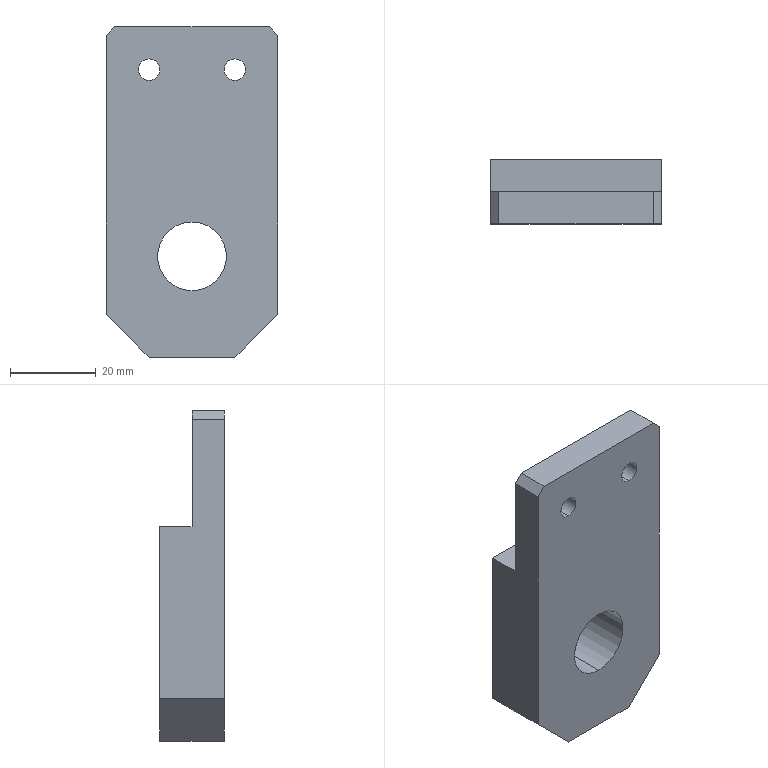Part | STEP file | 0229_219_Arm | 1 solid | 18 faces | box 40 x 15 x 77 mm | volume 33260 mm3 | plane 12 | cylinder 6 | commonest cylinder face diameters 5 x4 16 x2
STEP:
#1=CARTESIAN_POINT('',(0.,0.,0.));
#2=DIRECTION('',(0.,0.,1.));
#3=DIRECTION('',(1.,0.,0.));
#4=AXIS2_PLACEMENT_3D('',#1,#2,#3);
#5=CARTESIAN_POINT('',(-10.,0.,-7.5));
#6=VERTEX_POINT('',#5);
#7=CARTESIAN_POINT('',(-10.,7.5,-7.5));
#8=VERTEX_POINT('',#7);
#9=CARTESIAN_POINT('',(-10.,7.5,-7.5));
#10=DIRECTION('',(0.,1.,0.));
#11=VECTOR('',#10,1.);
#12=LINE('',#9,#11);
#13=CARTESIAN_POINT('',(-10.,7.5,-10.));
#14=DIRECTION('',(0.,1.,0.));
#15=DIRECTION('',(0.,0.,1.));
#16=AXIS2_PLACEMENT_3D('',#13,#14,#15);
#17=CYLINDRICAL_SURFACE('',#16,2.5);
#18=CARTESIAN_POINT('',(6.283,0.));
#19=DIRECTION('',(0.,1.));
#20=VECTOR('',#19,1.);
#21=LINE('',#18,#20);
#22=(GEOMETRIC_REPRESENTATION_CONTEXT(2)PARAMETRIC_REPRESENTATION_CONTEXT()REPRESENTATION_CONTEXT('',''));
#23=DEFINITIONAL_REPRESENTATION('',(#21),#22);
#24=PCURVE('',#17,#23);
#25=CARTESIAN_POINT('',(-10.,7.5,-10.));
#26=DIRECTION('',(0.,1.,0.));
#27=DIRECTION('',(0.,0.,1.));
#28=AXIS2_PLACEMENT_3D('',#25,#26,#27);
#29=CYLINDRICAL_SURFACE('',#28,2.5);
#30=CARTESIAN_POINT('',(0.,0.));
#31=DIRECTION('',(0.,1.));
#32=VECTOR('',#31,1.);
#33=LINE('',#30,#32);
#34=(GEOMETRIC_REPRESENTATION_CONTEXT(2)PARAMETRIC_REPRESENTATION_CONTEXT()REPRESENTATION_CONTEXT('',''));
#35=DEFINITIONAL_REPRESENTATION('',(#33),#34);
#36=PCURVE('',#29,#35);
#37=SURFACE_CURVE('',#12,(#24,#36),.PCURVE_S1.);
#38=EDGE_CURVE('',#6,#8,#37,.T.);
#39=ORIENTED_EDGE('',*,*,#38,.T.);
#40=CARTESIAN_POINT('',(-10.,7.5,-12.5));
#41=VERTEX_POINT('',#40);
#42=CARTESIAN_POINT('',(-10.,7.5,-10.));
#43=DIRECTION('',(0.,1.,0.));
#44=DIRECTION('',(0.,0.,1.));
#45=AXIS2_PLACEMENT_3D('',#42,#43,#44);
#46=CIRCLE('',#45,2.5);
#47=CARTESIAN_POINT('',(0.,0.));
#48=DIRECTION('',(1.,0.));
#49=VECTOR('',#48,1.);
#50=LINE('',#47,#49);
#51=(GEOMETRIC_REPRESENTATION_CONTEXT(2)PARAMETRIC_REPRESENTATION_CONTEXT()REPRESENTATION_CONTEXT('',''));
#52=DEFINITIONAL_REPRESENTATION('',(#50),#51);
#53=PCURVE('',#17,#52);
#54=CARTESIAN_POINT('',(-20.,7.5,-77.));
#55=DIRECTION('',(0.,-1.,0.));
#56=DIRECTION('',(0.,0.,-1.));
#57=AXIS2_PLACEMENT_3D('',#54,#55,#56);
#58=PLANE('',#57);
#59=CARTESIAN_POINT('',(-69.5,10.));
#60=CARTESIAN_POINT('',(-69.5,14.33));
#61=CARTESIAN_POINT('',(-65.75,12.165));
#62=CARTESIAN_POINT('',(-62.,10.));
#63=CARTESIAN_POINT('',(-65.75,7.835));
#64=CARTESIAN_POINT('',(-69.5,5.67));
#65=CARTESIAN_POINT('',(-69.5,10.));
#66=(BOUNDED_CURVE()B_SPLINE_CURVE(2,(#59,#60,#61,#62,#63,#64,#65),.UNSPECIFIED.,.T.,.F.)B_SPLINE_CURVE_WITH_KNOTS((1,2,2,2,2,1),(-2.094,0.,2.094,4.189,6.283,8.378),.UNSPECIFIED.)CURVE()GEOMETRIC_REPRESENTATION_ITEM()RATIONAL_B_SPLINE_CURVE((1.,0.5,1.,0.5,1.,0.5,1.))REPRESENTATION_ITEM(''));
#67=(GEOMETRIC_REPRESENTATION_CONTEXT(2)PARAMETRIC_REPRESENTATION_CONTEXT()REPRESENTATION_CONTEXT('',''));
#68=DEFINITIONAL_REPRESENTATION('',(#66),#67);
#69=PCURVE('',#58,#68);
#70=SURFACE_CURVE('',#46,(#53,#69),.PCURVE_S1.);
#71=EDGE_CURVE('',#41,#8,#70,.T.);
#72=ORIENTED_EDGE('',*,*,#71,.F.);
#73=CARTESIAN_POINT('',(-10.,0.,-12.5));
#74=VERTEX_POINT('',#73);
#75=CARTESIAN_POINT('',(-10.,7.5,-12.5));
#76=DIRECTION('',(0.,1.,0.));
#77=VECTOR('',#76,1.);
#78=LINE('',#75,#77);
#79=CARTESIAN_POINT('',(3.142,0.));
#80=DIRECTION('',(0.,1.));
#81=VECTOR('',#80,1.);
#82=LINE('',#79,#81);
#83=(GEOMETRIC_REPRESENTATION_CONTEXT(2)PARAMETRIC_REPRESENTATION_CONTEXT()REPRESENTATION_CONTEXT('',''));
#84=DEFINITIONAL_REPRESENTATION('',(#82),#83);
#85=PCURVE('',#17,#84);
#86=CARTESIAN_POINT('',(3.142,0.));
#87=DIRECTION('',(0.,1.));
#88=VECTOR('',#87,1.);
#89=LINE('',#86,#88);
#90=(GEOMETRIC_REPRESENTATION_CONTEXT(2)PARAMETRIC_REPRESENTATION_CONTEXT()REPRESENTATION_CONTEXT('',''));
#91=DEFINITIONAL_REPRESENTATION('',(#89),#90);
#92=PCURVE('',#29,#91);
#93=SURFACE_CURVE('',#78,(#85,#92),.PCURVE_S1.);
#94=EDGE_CURVE('',#74,#41,#93,.T.);
#95=ORIENTED_EDGE('',*,*,#94,.F.);
#96=CARTESIAN_POINT('',(-10.,0.,-10.));
#97=DIRECTION('',(0.,1.,0.));
#98=DIRECTION('',(0.,0.,1.));
#99=AXIS2_PLACEMENT_3D('',#96,#97,#98);
#100=CIRCLE('',#99,2.5);
#101=CARTESIAN_POINT('',(0.,-7.5));
#102=DIRECTION('',(1.,0.));
#103=VECTOR('',#102,1.);
#104=LINE('',#101,#103);
#105=(GEOMETRIC_REPRESENTATION_CONTEXT(2)PARAMETRIC_REPRESENTATION_CONTEXT()REPRESENTATION_CONTEXT('',''));
#106=DEFINITIONAL_REPRESENTATION('',(#104),#105);
#107=PCURVE('',#17,#106);
#108=CARTESIAN_POINT('',(-20.,0.,-77.));
#109=DIRECTION('',(0.,-1.,0.));
#110=DIRECTION('',(0.,0.,-1.));
#111=AXIS2_PLACEMENT_3D('',#108,#109,#110);
#112=PLANE('',#111);
#113=CARTESIAN_POINT('',(-69.5,10.));
#114=CARTESIAN_POINT('',(-69.5,14.33));
#115=CARTESIAN_POINT('',(-65.75,12.165));
#116=CARTESIAN_POINT('',(-62.,10.));
#117=CARTESIAN_POINT('',(-65.75,7.835));
#118=CARTESIAN_POINT('',(-69.5,5.67));
#119=CARTESIAN_POINT('',(-69.5,10.));
#120=(BOUNDED_CURVE()B_SPLINE_CURVE(2,(#113,#114,#115,#116,#117,#118,#119),.UNSPECIFIED.,.T.,.F.)B_SPLINE_CURVE_WITH_KNOTS((1,2,2,2,2,1),(-2.094,0.,2.094,4.189,6.283,8.378),.UNSPECIFIED.)CURVE()GEOMETRIC_REPRESENTATION_ITEM()RATIONAL_B_SPLINE_CURVE((1.,0.5,1.,0.5,1.,0.5,1.))REPRESENTATION_ITEM(''));
#121=(GEOMETRIC_REPRESENTATION_CONTEXT(2)PARAMETRIC_REPRESENTATION_CONTEXT()REPRESENTATION_CONTEXT('',''));
#122=DEFINITIONAL_REPRESENTATION('',(#120),#121);
#123=PCURVE('',#112,#122);
#124=SURFACE_CURVE('',#100,(#107,#123),.PCURVE_S1.);
#125=EDGE_CURVE('',#74,#6,#124,.T.);
#126=ORIENTED_EDGE('',*,*,#125,.T.);
#127=EDGE_LOOP('',(#39,#72,#95,#126));
#128=FACE_BOUND('',#127,.F.);
#129=ADVANCED_FACE('',(#128),#17,.F.);
#130=CARTESIAN_POINT('',(10.,0.,-7.5));
#131=VERTEX_POINT('',#130);
#132=CARTESIAN_POINT('',(10.,7.5,-7.5));
#133=VERTEX_POINT('',#132);
#134=CARTESIAN_POINT('',(10.,7.5,-7.5));
#135=DIRECTION('',(0.,1.,0.));
#136=VECTOR('',#135,1.);
#137=LINE('',#134,#136);
#138=CARTESIAN_POINT('',(10.,7.5,-10.));
#139=DIRECTION('',(0.,1.,0.));
#140=DIRECTION('',(0.,0.,1.));
#141=AXIS2_PLACEMENT_3D('',#138,#139,#140);
#142=CYLINDRICAL_SURFACE('',#141,2.5);
#143=CARTESIAN_POINT('',(6.283,0.));
#144=DIRECTION('',(0.,1.));
#145=VECTOR('',#144,1.);
#146=LINE('',#143,#145);
#147=(GEOMETRIC_REPRESENTATION_CONTEXT(2)PARAMETRIC_REPRESENTATION_CONTEXT()REPRESENTATION_CONTEXT('',''));
#148=DEFINITIONAL_REPRESENTATION('',(#146),#147);
#149=PCURVE('',#142,#148);
#150=CARTESIAN_POINT('',(10.,7.5,-10.));
#151=DIRECTION('',(0.,1.,0.));
#152=DIRECTION('',(0.,0.,1.));
#153=AXIS2_PLACEMENT_3D('',#150,#151,#152);
#154=CYLINDRICAL_SURFACE('',#153,2.5);
#155=CARTESIAN_POINT('',(0.,0.));
#156=DIRECTION('',(0.,1.));
#157=VECTOR('',#156,1.);
#158=LINE('',#155,#157);
#159=(GEOMETRIC_REPRESENTATION_CONTEXT(2)PARAMETRIC_REPRESENTATION_CONTEXT()REPRESENTATION_CONTEXT('',''));
#160=DEFINITIONAL_REPRESENTATION('',(#158),#159);
#161=PCURVE('',#154,#160);
#162=SURFACE_CURVE('',#137,(#149,#161),.PCURVE_S1.);
#163=EDGE_CURVE('',#131,#133,#162,.T.);
#164=ORIENTED_EDGE('',*,*,#163,.T.);
#165=CARTESIAN_POINT('',(10.,7.5,-12.5));
#166=VERTEX_POINT('',#165);
#167=CARTESIAN_POINT('',(10.,7.5,-10.));
#168=DIRECTION('',(0.,1.,0.));
#169=DIRECTION('',(0.,0.,1.));
#170=AXIS2_PLACEMENT_3D('',#167,#168,#169);
#171=CIRCLE('',#170,2.5);
#172=CARTESIAN_POINT('',(0.,0.));
#173=DIRECTION('',(1.,0.));
#174=VECTOR('',#173,1.);
#175=LINE('',#172,#174);
#176=(GEOMETRIC_REPRESENTATION_CONTEXT(2)PARAMETRIC_REPRESENTATION_CONTEXT()REPRESENTATION_CONTEXT('',''));
#177=DEFINITIONAL_REPRESENTATION('',(#175),#176);
#178=PCURVE('',#142,#177);
#179=CARTESIAN_POINT('',(-69.5,30.));
#180=CARTESIAN_POINT('',(-69.5,34.33));
#181=CARTESIAN_POINT('',(-65.75,32.165));
#182=CARTESIAN_POINT('',(-62.,30.));
#183=CARTESIAN_POINT('',(-65.75,27.835));
#184=CARTESIAN_POINT('',(-69.5,25.67));
#185=CARTESIAN_POINT('',(-69.5,30.));
#186=(BOUNDED_CURVE()B_SPLINE_CURVE(2,(#179,#180,#181,#182,#183,#184,#185),.UNSPECIFIED.,.T.,.F.)B_SPLINE_CURVE_WITH_KNOTS((1,2,2,2,2,1),(-2.094,0.,2.094,4.189,6.283,8.378),.UNSPECIFIED.)CURVE()GEOMETRIC_REPRESENTATION_ITEM()RATIONAL_B_SPLINE_CURVE((1.,0.5,1.,0.5,1.,0.5,1.))REPRESENTATION_ITEM(''));
#187=(GEOMETRIC_REPRESENTATION_CONTEXT(2)PARAMETRIC_REPRESENTATION_CONTEXT()REPRESENTATION_CONTEXT('',''));
#188=DEFINITIONAL_REPRESENTATION('',(#186),#187);
#189=PCURVE('',#58,#188);
#190=SURFACE_CURVE('',#171,(#178,#189),.PCURVE_S1.);
#191=EDGE_CURVE('',#166,#133,#190,.T.);
#192=ORIENTED_EDGE('',*,*,#191,.F.);
#193=CARTESIAN_POINT('',(10.,0.,-12.5));
#194=VERTEX_POINT('',#193);
#195=CARTESIAN_POINT('',(10.,7.5,-12.5));
#196=DIRECTION('',(0.,1.,0.));
#197=VECTOR('',#196,1.);
#198=LINE('',#195,#197);
#199=CARTESIAN_POINT('',(3.142,0.));
#200=DIRECTION('',(0.,1.));
#201=VECTOR('',#200,1.);
#202=LINE('',#199,#201);
#203=(GEOMETRIC_REPRESENTATION_CONTEXT(2)PARAMETRIC_REPRESENTATION_CONTEXT()REPRESENTATION_CONTEXT('',''));
#204=DEFINITIONAL_REPRESENTATION('',(#202),#203);
#205=PCURVE('',#142,#204);
#206=CARTESIAN_POINT('',(3.142,0.));
#207=DIRECTION('',(0.,1.));
#208=VECTOR('',#207,1.);
#209=LINE('',#206,#208);
#210=(GEOMETRIC_REPRESENTATION_CONTEXT(2)PARAMETRIC_REPRESENTATION_CONTEXT()REPRESENTATION_CONTEXT('',''));
#211=DEFINITIONAL_REPRESENTATION('',(#209),#210);
#212=PCURVE('',#154,#211);
#213=SURFACE_CURVE('',#198,(#205,#212),.PCURVE_S1.);
#214=EDGE_CURVE('',#194,#166,#213,.T.);
#215=ORIENTED_EDGE('',*,*,#214,.F.);
#216=CARTESIAN_POINT('',(10.,0.,-10.));
#217=DIRECTION('',(0.,1.,0.));
#218=DIRECTION('',(0.,0.,1.));
#219=AXIS2_PLACEMENT_3D('',#216,#217,#218);
#220=CIRCLE('',#219,2.5);
#221=CARTESIAN_POINT('',(0.,-7.5));
#222=DIRECTION('',(1.,0.));
#223=VECTOR('',#222,1.);
#224=LINE('',#221,#223);
#225=(GEOMETRIC_REPRESENTATION_CONTEXT(2)PARAMETRIC_REPRESENTATION_CONTEXT()REPRESENTATION_CONTEXT('',''));
#226=DEFINITIONAL_REPRESENTATION('',(#224),#225);
#227=PCURVE('',#142,#226);
#228=CARTESIAN_POINT('',(-69.5,30.));
#229=CARTESIAN_POINT('',(-69.5,34.33));
#230=CARTESIAN_POINT('',(-65.75,32.165));
#231=CARTESIAN_POINT('',(-62.,30.));
#232=CARTESIAN_POINT('',(-65.75,27.835));
#233=CARTESIAN_POINT('',(-69.5,25.67));
#234=CARTESIAN_POINT('',(-69.5,30.));
#235=(BOUNDED_CURVE()B_SPLINE_CURVE(2,(#228,#229,#230,#231,#232,#233,#234),.UNSPECIFIED.,.T.,.F.)B_SPLINE_CURVE_WITH_KNOTS((1,2,2,2,2,1),(-2.094,0.,2.094,4.189,6.283,8.378),.UNSPECIFIED.)CURVE()GEOMETRIC_REPRESENTATION_ITEM()RATIONAL_B_SPLINE_CURVE((1.,0.5,1.,0.5,1.,0.5,1.))REPRESENTATION_ITEM(''));
#236=(GEOMETRIC_REPRESENTATION_CONTEXT(2)PARAMETRIC_REPRESENTATION_CONTEXT()REPRESENTATION_CONTEXT('',''));
#237=DEFINITIONAL_REPRESENTATION('',(#235),#236);
#238=PCURVE('',#112,#237);
#239=SURFACE_CURVE('',#220,(#227,#238),.PCURVE_S1.);
#240=EDGE_CURVE('',#194,#131,#239,.T.);
#241=ORIENTED_EDGE('',*,*,#240,.T.);
#242=EDGE_LOOP('',(#164,#192,#215,#241));
#243=FACE_BOUND('',#242,.F.);
#244=ADVANCED_FACE('',(#243),#142,.F.);
#245=CARTESIAN_POINT('',(0.,0.,-45.5));
#246=VERTEX_POINT('',#245);
#247=CARTESIAN_POINT('',(0.,15.,-45.5));
#248=VERTEX_POINT('',#247);
#249=CARTESIAN_POINT('',(0.,0.,-45.5));
#250=DIRECTION('',(0.,1.,0.));
#251=VECTOR('',#250,1.);
#252=LINE('',#249,#251);
#253=CARTESIAN_POINT('',(0.,0.,-53.5));
#254=DIRECTION('',(0.,1.,0.));
#255=DIRECTION('',(0.,0.,1.));
#256=AXIS2_PLACEMENT_3D('',#253,#254,#255);
#257=CYLINDRICAL_SURFACE('',#256,8.);
#258=CARTESIAN_POINT('',(6.283,0.));
#259=DIRECTION('',(0.,1.));
#260=VECTOR('',#259,1.);
#261=LINE('',#258,#260);
#262=(GEOMETRIC_REPRESENTATION_CONTEXT(2)PARAMETRIC_REPRESENTATION_CONTEXT()REPRESENTATION_CONTEXT('',''));
#263=DEFINITIONAL_REPRESENTATION('',(#261),#262);
#264=PCURVE('',#257,#263);
#265=CARTESIAN_POINT('',(0.,0.,-53.5));
#266=DIRECTION('',(0.,1.,0.));
#267=DIRECTION('',(0.,0.,1.));
#268=AXIS2_PLACEMENT_3D('',#265,#266,#267);
#269=CYLINDRICAL_SURFACE('',#268,8.);
#270=CARTESIAN_POINT('',(0.,0.));
#271=DIRECTION('',(0.,1.));
#272=VECTOR('',#271,1.);
#273=LINE('',#270,#272);
#274=(GEOMETRIC_REPRESENTATION_CONTEXT(2)PARAMETRIC_REPRESENTATION_CONTEXT()REPRESENTATION_CONTEXT('',''));
#275=DEFINITIONAL_REPRESENTATION('',(#273),#274);
#276=PCURVE('',#269,#275);
#277=SURFACE_CURVE('',#252,(#264,#276),.PCURVE_S1.);
#278=EDGE_CURVE('',#246,#248,#277,.T.);
#279=ORIENTED_EDGE('',*,*,#278,.T.);
#280=CARTESIAN_POINT('',(0.,15.,-61.5));
#281=VERTEX_POINT('',#280);
#282=CARTESIAN_POINT('',(0.,15.,-53.5));
#283=DIRECTION('',(0.,1.,0.));
#284=DIRECTION('',(0.,0.,1.));
#285=AXIS2_PLACEMENT_3D('',#282,#283,#284);
#286=CIRCLE('',#285,8.);
#287=CARTESIAN_POINT('',(0.,15.));
#288=DIRECTION('',(1.,0.));
#289=VECTOR('',#288,1.);
#290=LINE('',#287,#289);
#291=(GEOMETRIC_REPRESENTATION_CONTEXT(2)PARAMETRIC_REPRESENTATION_CONTEXT()REPRESENTATION_CONTEXT('',''));
#292=DEFINITIONAL_REPRESENTATION('',(#290),#291);
#293=PCURVE('',#257,#292);
#294=CARTESIAN_POINT('',(-20.,15.,-77.));
#295=DIRECTION('',(0.,-1.,0.));
#296=DIRECTION('',(0.,0.,-1.));
#297=AXIS2_PLACEMENT_3D('',#294,#295,#296);
#298=PLANE('',#297);
#299=CARTESIAN_POINT('',(-31.5,20.));
#300=CARTESIAN_POINT('',(-31.5,33.856));
#301=CARTESIAN_POINT('',(-19.5,26.928));
#302=CARTESIAN_POINT('',(-7.5,20.));
#303=CARTESIAN_POINT('',(-19.5,13.072));
#304=CARTESIAN_POINT('',(-31.5,6.144));
#305=CARTESIAN_POINT('',(-31.5,20.));
#306=(BOUNDED_CURVE()B_SPLINE_CURVE(2,(#299,#300,#301,#302,#303,#304,#305),.UNSPECIFIED.,.T.,.F.)B_SPLINE_CURVE_WITH_KNOTS((1,2,2,2,2,1),(-2.094,0.,2.094,4.189,6.283,8.378),.UNSPECIFIED.)CURVE()GEOMETRIC_REPRESENTATION_ITEM()RATIONAL_B_SPLINE_CURVE((1.,0.5,1.,0.5,1.,0.5,1.))REPRESENTATION_ITEM(''));
#307=(GEOMETRIC_REPRESENTATION_CONTEXT(2)PARAMETRIC_REPRESENTATION_CONTEXT()REPRESENTATION_CONTEXT('',''));
#308=DEFINITIONAL_REPRESENTATION('',(#306),#307);
#309=PCURVE('',#298,#308);
#310=SURFACE_CURVE('',#286,(#293,#309),.PCURVE_S1.);
#311=EDGE_CURVE('',#281,#248,#310,.T.);
#312=ORIENTED_EDGE('',*,*,#311,.F.);
#313=CARTESIAN_POINT('',(0.,0.,-61.5));
#314=VERTEX_POINT('',#313);
#315=CARTESIAN_POINT('',(0.,0.,-61.5));
#316=DIRECTION('',(0.,1.,0.));
#317=VECTOR('',#316,1.);
#318=LINE('',#315,#317);
#319=CARTESIAN_POINT('',(3.142,0.));
#320=DIRECTION('',(0.,1.));
#321=VECTOR('',#320,1.);
#322=LINE('',#319,#321);
#323=(GEOMETRIC_REPRESENTATION_CONTEXT(2)PARAMETRIC_REPRESENTATION_CONTEXT()REPRESENTATION_CONTEXT('',''));
#324=DEFINITIONAL_REPRESENTATION('',(#322),#323);
#325=PCURVE('',#257,#324);
#326=CARTESIAN_POINT('',(3.142,0.));
#327=DIRECTION('',(0.,1.));
#328=VECTOR('',#327,1.);
#329=LINE('',#326,#328);
#330=(GEOMETRIC_REPRESENTATION_CONTEXT(2)PARAMETRIC_REPRESENTATION_CONTEXT()REPRESENTATION_CONTEXT('',''));
#331=DEFINITIONAL_REPRESENTATION('',(#329),#330);
#332=PCURVE('',#269,#331);
#333=SURFACE_CURVE('',#318,(#325,#332),.PCURVE_S1.);
#334=EDGE_CURVE('',#314,#281,#333,.T.);
#335=ORIENTED_EDGE('',*,*,#334,.F.);
#336=CARTESIAN_POINT('',(0.,0.,-53.5));
#337=DIRECTION('',(0.,1.,0.));
#338=DIRECTION('',(0.,0.,1.));
#339=AXIS2_PLACEMENT_3D('',#336,#337,#338);
#340=CIRCLE('',#339,8.);
#341=CARTESIAN_POINT('',(0.,0.));
#342=DIRECTION('',(1.,0.));
#343=VECTOR('',#342,1.);
#344=LINE('',#341,#343);
#345=(GEOMETRIC_REPRESENTATION_CONTEXT(2)PARAMETRIC_REPRESENTATION_CONTEXT()REPRESENTATION_CONTEXT('',''));
#346=DEFINITIONAL_REPRESENTATION('',(#344),#345);
#347=PCURVE('',#257,#346);
#348=CARTESIAN_POINT('',(-31.5,20.));
#349=CARTESIAN_POINT('',(-31.5,33.856));
#350=CARTESIAN_POINT('',(-19.5,26.928));
#351=CARTESIAN_POINT('',(-7.5,20.));
#352=CARTESIAN_POINT('',(-19.5,13.072));
#353=CARTESIAN_POINT('',(-31.5,6.144));
#354=CARTESIAN_POINT('',(-31.5,20.));
#355=(BOUNDED_CURVE()B_SPLINE_CURVE(2,(#348,#349,#350,#351,#352,#353,#354),.UNSPECIFIED.,.T.,.F.)B_SPLINE_CURVE_WITH_KNOTS((1,2,2,2,2,1),(-2.094,0.,2.094,4.189,6.283,8.378),.UNSPECIFIED.)CURVE()GEOMETRIC_REPRESENTATION_ITEM()RATIONAL_B_SPLINE_CURVE((1.,0.5,1.,0.5,1.,0.5,1.))REPRESENTATION_ITEM(''));
#356=(GEOMETRIC_REPRESENTATION_CONTEXT(2)PARAMETRIC_REPRESENTATION_CONTEXT()REPRESENTATION_CONTEXT('',''));
#357=DEFINITIONAL_REPRESENTATION('',(#355),#356);
#358=PCURVE('',#112,#357);
#359=SURFACE_CURVE('',#340,(#347,#358),.PCURVE_S1.);
#360=EDGE_CURVE('',#314,#246,#359,.T.);
#361=ORIENTED_EDGE('',*,*,#360,.T.);
#362=EDGE_LOOP('',(#279,#312,#335,#361));
#363=FACE_BOUND('',#362,.F.);
#364=ADVANCED_FACE('',(#363),#257,.F.);
#365=CARTESIAN_POINT('',(-20.,0.,-67.));
#366=VERTEX_POINT('',#365);
#367=CARTESIAN_POINT('',(-20.,0.,-2.));
#368=VERTEX_POINT('',#367);
#369=CARTESIAN_POINT('',(-20.,0.,0.));
#370=DIRECTION('',(0.,0.,1.));
#371=VECTOR('',#370,1.);
#372=LINE('',#369,#371);
#373=CARTESIAN_POINT('',(-20.,15.,0.));
#374=DIRECTION('',(1.,0.,0.));
#375=DIRECTION('',(0.,0.,-1.));
#376=AXIS2_PLACEMENT_3D('',#373,#374,#375);
#377=PLANE('',#376);
#378=CARTESIAN_POINT('',(0.,-15.));
#379=DIRECTION('',(-1.,0.));
#380=VECTOR('',#379,1.);
#381=LINE('',#378,#380);
#382=(GEOMETRIC_REPRESENTATION_CONTEXT(2)PARAMETRIC_REPRESENTATION_CONTEXT()REPRESENTATION_CONTEXT('',''));
#383=DEFINITIONAL_REPRESENTATION('',(#381),#382);
#384=PCURVE('',#377,#383);
#385=CARTESIAN_POINT('',(-77.,0.));
#386=DIRECTION('',(-1.,0.));
#387=VECTOR('',#386,1.);
#388=LINE('',#385,#387);
#389=(GEOMETRIC_REPRESENTATION_CONTEXT(2)PARAMETRIC_REPRESENTATION_CONTEXT()REPRESENTATION_CONTEXT('',''));
#390=DEFINITIONAL_REPRESENTATION('',(#388),#389);
#391=PCURVE('',#112,#390);
#392=SURFACE_CURVE('',#372,(#384,#391),.PCURVE_S1.);
#393=EDGE_CURVE('',#366,#368,#392,.T.);
#394=ORIENTED_EDGE('',*,*,#393,.T.);
#395=CARTESIAN_POINT('',(-20.,7.5,-2.));
#396=VERTEX_POINT('',#395);
#397=CARTESIAN_POINT('',(-20.,15.,-2.));
#398=DIRECTION('',(0.,1.,0.));
#399=VECTOR('',#398,1.);
#400=LINE('',#397,#399);
#401=CARTESIAN_POINT('',(2.,0.));
#402=DIRECTION('',(0.,1.));
#403=VECTOR('',#402,1.);
#404=LINE('',#401,#403);
#405=(GEOMETRIC_REPRESENTATION_CONTEXT(2)PARAMETRIC_REPRESENTATION_CONTEXT()REPRESENTATION_CONTEXT('',''));
#406=DEFINITIONAL_REPRESENTATION('',(#404),#405);
#407=PCURVE('',#377,#406);
#408=CARTESIAN_POINT('',(-18.,15.,0.));
#409=DIRECTION('',(0.7071,0.,-0.7071));
#410=DIRECTION('',(-0.7071,0.,-0.7071));
#411=AXIS2_PLACEMENT_3D('',#408,#409,#410);
#412=PLANE('',#411);
#413=CARTESIAN_POINT('',(2.828,0.));
#414=DIRECTION('',(0.,1.));
#415=VECTOR('',#414,1.);
#416=LINE('',#413,#415);
#417=(GEOMETRIC_REPRESENTATION_CONTEXT(2)PARAMETRIC_REPRESENTATION_CONTEXT()REPRESENTATION_CONTEXT('',''));
#418=DEFINITIONAL_REPRESENTATION('',(#416),#417);
#419=PCURVE('',#412,#418);
#420=SURFACE_CURVE('',#400,(#407,#419),.PCURVE_S1.);
#421=EDGE_CURVE('',#368,#396,#420,.T.);
#422=ORIENTED_EDGE('',*,*,#421,.T.);
#423=CARTESIAN_POINT('',(-20.,7.5,-27.));
#424=VERTEX_POINT('',#423);
#425=CARTESIAN_POINT('',(-20.,7.5,0.));
#426=DIRECTION('',(0.,0.,1.));
#427=VECTOR('',#426,1.);
#428=LINE('',#425,#427);
#429=CARTESIAN_POINT('',(0.,-7.5));
#430=DIRECTION('',(-1.,0.));
#431=VECTOR('',#430,1.);
#432=LINE('',#429,#431);
#433=(GEOMETRIC_REPRESENTATION_CONTEXT(2)PARAMETRIC_REPRESENTATION_CONTEXT()REPRESENTATION_CONTEXT('',''));
#434=DEFINITIONAL_REPRESENTATION('',(#432),#433);
#435=PCURVE('',#377,#434);
#436=CARTESIAN_POINT('',(-77.,0.));
#437=DIRECTION('',(-1.,0.));
#438=VECTOR('',#437,1.);
#439=LINE('',#436,#438);
#440=(GEOMETRIC_REPRESENTATION_CONTEXT(2)PARAMETRIC_REPRESENTATION_CONTEXT()REPRESENTATION_CONTEXT('',''));
#441=DEFINITIONAL_REPRESENTATION('',(#439),#440);
#442=PCURVE('',#58,#441);
#443=SURFACE_CURVE('',#428,(#435,#442),.PCURVE_S1.);
#444=EDGE_CURVE('',#424,#396,#443,.T.);
#445=ORIENTED_EDGE('',*,*,#444,.F.);
#446=CARTESIAN_POINT('',(-20.,15.,-27.));
#447=VERTEX_POINT('',#446);
#448=CARTESIAN_POINT('',(-20.,-48.26,-27.));
#449=DIRECTION('',(0.,1.,0.));
#450=VECTOR('',#449,1.);
#451=LINE('',#448,#450);
#452=CARTESIAN_POINT('',(27.,-63.26));
#453=DIRECTION('',(0.,1.));
#454=VECTOR('',#453,1.);
#455=LINE('',#452,#454);
#456=(GEOMETRIC_REPRESENTATION_CONTEXT(2)PARAMETRIC_REPRESENTATION_CONTEXT()REPRESENTATION_CONTEXT('',''));
#457=DEFINITIONAL_REPRESENTATION('',(#455),#456);
#458=PCURVE('',#377,#457);
#459=CARTESIAN_POINT('',(-20.,-48.26,-27.));
#460=DIRECTION('',(0.,0.,-1.));
#461=DIRECTION('',(-1.,0.,0.));
#462=AXIS2_PLACEMENT_3D('',#459,#460,#461);
#463=PLANE('',#462);
#464=CARTESIAN_POINT('',(0.,0.));
#465=DIRECTION('',(0.,1.));
#466=VECTOR('',#465,1.);
#467=LINE('',#464,#466);
#468=(GEOMETRIC_REPRESENTATION_CONTEXT(2)PARAMETRIC_REPRESENTATION_CONTEXT()REPRESENTATION_CONTEXT('',''));
#469=DEFINITIONAL_REPRESENTATION('',(#467),#468);
#470=PCURVE('',#463,#469);
#471=SURFACE_CURVE('',#451,(#458,#470),.PCURVE_S1.);
#472=EDGE_CURVE('',#424,#447,#471,.T.);
#473=ORIENTED_EDGE('',*,*,#472,.T.);
#474=CARTESIAN_POINT('',(-20.,15.,-67.));
#475=VERTEX_POINT('',#474);
#476=CARTESIAN_POINT('',(-20.,15.,0.));
#477=DIRECTION('',(0.,0.,1.));
#478=VECTOR('',#477,1.);
#479=LINE('',#476,#478);
#480=CARTESIAN_POINT('',(0.,0.));
#481=DIRECTION('',(-1.,0.));
#482=VECTOR('',#481,1.);
#483=LINE('',#480,#482);
#484=(GEOMETRIC_REPRESENTATION_CONTEXT(2)PARAMETRIC_REPRESENTATION_CONTEXT()REPRESENTATION_CONTEXT('',''));
#485=DEFINITIONAL_REPRESENTATION('',(#483),#484);
#486=PCURVE('',#377,#485);
#487=CARTESIAN_POINT('',(-77.,0.));
#488=DIRECTION('',(-1.,0.));
#489=VECTOR('',#488,1.);
#490=LINE('',#487,#489);
#491=(GEOMETRIC_REPRESENTATION_CONTEXT(2)PARAMETRIC_REPRESENTATION_CONTEXT()REPRESENTATION_CONTEXT('',''));
#492=DEFINITIONAL_REPRESENTATION('',(#490),#491);
#493=PCURVE('',#298,#492);
#494=SURFACE_CURVE('',#479,(#486,#493),.PCURVE_S1.);
#495=EDGE_CURVE('',#475,#447,#494,.T.);
#496=ORIENTED_EDGE('',*,*,#495,.F.);
#497=CARTESIAN_POINT('',(-20.,15.,-67.));
#498=DIRECTION('',(0.,-1.,0.));
#499=VECTOR('',#498,1.);
#500=LINE('',#497,#499);
#501=CARTESIAN_POINT('',(67.,0.));
#502=DIRECTION('',(0.,-1.));
#503=VECTOR('',#502,1.);
#504=LINE('',#501,#503);
#505=(GEOMETRIC_REPRESENTATION_CONTEXT(2)PARAMETRIC_REPRESENTATION_CONTEXT()REPRESENTATION_CONTEXT('',''));
#506=DEFINITIONAL_REPRESENTATION('',(#504),#505);
#507=PCURVE('',#377,#506);
#508=CARTESIAN_POINT('',(-20.,15.,-67.));
#509=DIRECTION('',(0.7071,0.,0.7071));
#510=DIRECTION('',(0.7071,0.,-0.7071));
#511=AXIS2_PLACEMENT_3D('',#508,#509,#510);
#512=PLANE('',#511);
#513=CARTESIAN_POINT('',(0.,0.));
#514=DIRECTION('',(0.,-1.));
#515=VECTOR('',#514,1.);
#516=LINE('',#513,#515);
#517=(GEOMETRIC_REPRESENTATION_CONTEXT(2)PARAMETRIC_REPRESENTATION_CONTEXT()REPRESENTATION_CONTEXT('',''));
#518=DEFINITIONAL_REPRESENTATION('',(#516),#517);
#519=PCURVE('',#512,#518);
#520=SURFACE_CURVE('',#500,(#507,#519),.PCURVE_S1.);
#521=EDGE_CURVE('',#475,#366,#520,.T.);
#522=ORIENTED_EDGE('',*,*,#521,.T.);
#523=EDGE_LOOP('',(#394,#422,#445,#473,#496,#522));
#524=FACE_BOUND('',#523,.T.);
#525=ADVANCED_FACE('',(#524),#377,.F.);
#526=CARTESIAN_POINT('',(-18.,0.,0.));
#527=VERTEX_POINT('',#526);
#528=CARTESIAN_POINT('',(18.,0.,0.));
#529=VERTEX_POINT('',#528);
#530=CARTESIAN_POINT('',(-20.,0.,0.));
#531=DIRECTION('',(1.,0.,0.));
#532=VECTOR('',#531,1.);
#533=LINE('',#530,#532);
#534=CARTESIAN_POINT('',(-20.,15.,0.));
#535=DIRECTION('',(0.,0.,-1.));
#536=DIRECTION('',(-1.,0.,0.));
#537=AXIS2_PLACEMENT_3D('',#534,#535,#536);
#538=PLANE('',#537);
#539=CARTESIAN_POINT('',(0.,-15.));
#540=DIRECTION('',(-1.,0.));
#541=VECTOR('',#540,1.);
#542=LINE('',#539,#541);
#543=(GEOMETRIC_REPRESENTATION_CONTEXT(2)PARAMETRIC_REPRESENTATION_CONTEXT()REPRESENTATION_CONTEXT('',''));
#544=DEFINITIONAL_REPRESENTATION('',(#542),#543);
#545=PCURVE('',#538,#544);
#546=CARTESIAN_POINT('',(-77.,0.));
#547=DIRECTION('',(0.,1.));
#548=VECTOR('',#547,1.);
#549=LINE('',#546,#548);
#550=(GEOMETRIC_REPRESENTATION_CONTEXT(2)PARAMETRIC_REPRESENTATION_CONTEXT()REPRESENTATION_CONTEXT('',''));
#551=DEFINITIONAL_REPRESENTATION('',(#549),#550);
#552=PCURVE('',#112,#551);
#553=SURFACE_CURVE('',#533,(#545,#552),.PCURVE_S1.);
#554=EDGE_CURVE('',#527,#529,#553,.T.);
#555=ORIENTED_EDGE('',*,*,#554,.T.);
#556=CARTESIAN_POINT('',(18.,7.5,0.));
#557=VERTEX_POINT('',#556);
#558=CARTESIAN_POINT('',(18.,15.,0.));
#559=DIRECTION('',(0.,1.,0.));
#560=VECTOR('',#559,1.);
#561=LINE('',#558,#560);
#562=CARTESIAN_POINT('',(-38.,0.));
#563=DIRECTION('',(0.,1.));
#564=VECTOR('',#563,1.);
#565=LINE('',#562,#564);
#566=(GEOMETRIC_REPRESENTATION_CONTEXT(2)PARAMETRIC_REPRESENTATION_CONTEXT()REPRESENTATION_CONTEXT('',''));
#567=DEFINITIONAL_REPRESENTATION('',(#565),#566);
#568=PCURVE('',#538,#567);
#569=CARTESIAN_POINT('',(20.,15.,-2.));
#570=DIRECTION('',(-0.7071,0.,-0.7071));
#571=DIRECTION('',(-0.7071,0.,0.7071));
#572=AXIS2_PLACEMENT_3D('',#569,#570,#571);
#573=PLANE('',#572);
#574=CARTESIAN_POINT('',(2.828,0.));
#575=DIRECTION('',(0.,1.));
#576=VECTOR('',#575,1.);
#577=LINE('',#574,#576);
#578=(GEOMETRIC_REPRESENTATION_CONTEXT(2)PARAMETRIC_REPRESENTATION_CONTEXT()REPRESENTATION_CONTEXT('',''));
#579=DEFINITIONAL_REPRESENTATION('',(#577),#578);
#580=PCURVE('',#573,#579);
#581=SURFACE_CURVE('',#561,(#568,#580),.PCURVE_S1.);
#582=EDGE_CURVE('',#529,#557,#581,.T.);
#583=ORIENTED_EDGE('',*,*,#582,.T.);
#584=CARTESIAN_POINT('',(-18.,7.5,0.));
#585=VERTEX_POINT('',#584);
#586=CARTESIAN_POINT('',(-20.,7.5,0.));
#587=DIRECTION('',(1.,0.,0.));
#588=VECTOR('',#587,1.);
#589=LINE('',#586,#588);
#590=CARTESIAN_POINT('',(0.,-7.5));
#591=DIRECTION('',(-1.,0.));
#592=VECTOR('',#591,1.);
#593=LINE('',#590,#592);
#594=(GEOMETRIC_REPRESENTATION_CONTEXT(2)PARAMETRIC_REPRESENTATION_CONTEXT()REPRESENTATION_CONTEXT('',''));
#595=DEFINITIONAL_REPRESENTATION('',(#593),#594);
#596=PCURVE('',#538,#595);
#597=CARTESIAN_POINT('',(-77.,0.));
#598=DIRECTION('',(0.,1.));
#599=VECTOR('',#598,1.);
#600=LINE('',#597,#599);
#601=(GEOMETRIC_REPRESENTATION_CONTEXT(2)PARAMETRIC_REPRESENTATION_CONTEXT()REPRESENTATION_CONTEXT('',''));
#602=DEFINITIONAL_REPRESENTATION('',(#600),#601);
#603=PCURVE('',#58,#602);
#604=SURFACE_CURVE('',#589,(#596,#603),.PCURVE_S1.);
#605=EDGE_CURVE('',#585,#557,#604,.T.);
#606=ORIENTED_EDGE('',*,*,#605,.F.);
#607=CARTESIAN_POINT('',(-18.,15.,0.));
#608=DIRECTION('',(0.,-1.,0.));
#609=VECTOR('',#608,1.);
#610=LINE('',#607,#609);
#611=CARTESIAN_POINT('',(-2.,0.));
#612=DIRECTION('',(0.,-1.));
#613=VECTOR('',#612,1.);
#614=LINE('',#611,#613);
#615=(GEOMETRIC_REPRESENTATION_CONTEXT(2)PARAMETRIC_REPRESENTATION_CONTEXT()REPRESENTATION_CONTEXT('',''));
#616=DEFINITIONAL_REPRESENTATION('',(#614),#615);
#617=PCURVE('',#538,#616);
#618=CARTESIAN_POINT('',(0.,0.));
#619=DIRECTION('',(0.,-1.));
#620=VECTOR('',#619,1.);
#621=LINE('',#618,#620);
#622=(GEOMETRIC_REPRESENTATION_CONTEXT(2)PARAMETRIC_REPRESENTATION_CONTEXT()REPRESENTATION_CONTEXT('',''));
#623=DEFINITIONAL_REPRESENTATION('',(#621),#622);
#624=PCURVE('',#412,#623);
#625=SURFACE_CURVE('',#610,(#617,#624),.PCURVE_S1.);
#626=EDGE_CURVE('',#585,#527,#625,.T.);
#627=ORIENTED_EDGE('',*,*,#626,.T.);
#628=EDGE_LOOP('',(#555,#583,#606,#627));
#629=FACE_BOUND('',#628,.T.);
#630=ADVANCED_FACE('',(#629),#538,.F.);
#631=CARTESIAN_POINT('',(20.,7.5,-2.));
#632=VERTEX_POINT('',#631);
#633=CARTESIAN_POINT('',(20.,7.5,-27.));
#634=VERTEX_POINT('',#633);
#635=CARTESIAN_POINT('',(20.,7.5,0.));
#636=DIRECTION('',(0.,0.,-1.));
#637=VECTOR('',#636,1.);
#638=LINE('',#635,#637);
#639=CARTESIAN_POINT('',(20.,15.,0.));
#640=DIRECTION('',(-1.,0.,0.));
#641=DIRECTION('',(0.,0.,1.));
#642=AXIS2_PLACEMENT_3D('',#639,#640,#641);
#643=PLANE('',#642);
#644=CARTESIAN_POINT('',(0.,-7.5));
#645=DIRECTION('',(-1.,0.));
#646=VECTOR('',#645,1.);
#647=LINE('',#644,#646);
#648=(GEOMETRIC_REPRESENTATION_CONTEXT(2)PARAMETRIC_REPRESENTATION_CONTEXT()REPRESENTATION_CONTEXT('',''));
#649=DEFINITIONAL_REPRESENTATION('',(#647),#648);
#650=PCURVE('',#643,#649);
#651=CARTESIAN_POINT('',(-77.,40.));
#652=DIRECTION('',(1.,0.));
#653=VECTOR('',#652,1.);
#654=LINE('',#651,#653);
#655=(GEOMETRIC_REPRESENTATION_CONTEXT(2)PARAMETRIC_REPRESENTATION_CONTEXT()REPRESENTATION_CONTEXT('',''));
#656=DEFINITIONAL_REPRESENTATION('',(#654),#655);
#657=PCURVE('',#58,#656);
#658=SURFACE_CURVE('',#638,(#650,#657),.PCURVE_S1.);
#659=EDGE_CURVE('',#632,#634,#658,.T.);
#660=ORIENTED_EDGE('',*,*,#659,.F.);
#661=CARTESIAN_POINT('',(20.,0.,-2.));
#662=VERTEX_POINT('',#661);
#663=CARTESIAN_POINT('',(20.,15.,-2.));
#664=DIRECTION('',(0.,-1.,0.));
#665=VECTOR('',#664,1.);
#666=LINE('',#663,#665);
#667=CARTESIAN_POINT('',(-2.,0.));
#668=DIRECTION('',(0.,-1.));
#669=VECTOR('',#668,1.);
#670=LINE('',#667,#669);
#671=(GEOMETRIC_REPRESENTATION_CONTEXT(2)PARAMETRIC_REPRESENTATION_CONTEXT()REPRESENTATION_CONTEXT('',''));
#672=DEFINITIONAL_REPRESENTATION('',(#670),#671);
#673=PCURVE('',#643,#672);
#674=CARTESIAN_POINT('',(0.,0.));
#675=DIRECTION('',(0.,-1.));
#676=VECTOR('',#675,1.);
#677=LINE('',#674,#676);
#678=(GEOMETRIC_REPRESENTATION_CONTEXT(2)PARAMETRIC_REPRESENTATION_CONTEXT()REPRESENTATION_CONTEXT('',''));
#679=DEFINITIONAL_REPRESENTATION('',(#677),#678);
#680=PCURVE('',#573,#679);
#681=SURFACE_CURVE('',#666,(#673,#680),.PCURVE_S1.);
#682=EDGE_CURVE('',#632,#662,#681,.T.);
#683=ORIENTED_EDGE('',*,*,#682,.T.);
#684=CARTESIAN_POINT('',(20.,0.,-67.));
#685=VERTEX_POINT('',#684);
#686=CARTESIAN_POINT('',(20.,0.,0.));
#687=DIRECTION('',(0.,0.,-1.));
#688=VECTOR('',#687,1.);
#689=LINE('',#686,#688);
#690=CARTESIAN_POINT('',(0.,-15.));
#691=DIRECTION('',(-1.,0.));
#692=VECTOR('',#691,1.);
#693=LINE('',#690,#692);
#694=(GEOMETRIC_REPRESENTATION_CONTEXT(2)PARAMETRIC_REPRESENTATION_CONTEXT()REPRESENTATION_CONTEXT('',''));
#695=DEFINITIONAL_REPRESENTATION('',(#693),#694);
#696=PCURVE('',#643,#695);
#697=CARTESIAN_POINT('',(-77.,40.));
#698=DIRECTION('',(1.,0.));
#699=VECTOR('',#698,1.);
#700=LINE('',#697,#699);
#701=(GEOMETRIC_REPRESENTATION_CONTEXT(2)PARAMETRIC_REPRESENTATION_CONTEXT()REPRESENTATION_CONTEXT('',''));
#702=DEFINITIONAL_REPRESENTATION('',(#700),#701);
#703=PCURVE('',#112,#702);
#704=SURFACE_CURVE('',#689,(#696,#703),.PCURVE_S1.);
#705=EDGE_CURVE('',#662,#685,#704,.T.);
#706=ORIENTED_EDGE('',*,*,#705,.T.);
#707=CARTESIAN_POINT('',(20.,15.,-67.));
#708=VERTEX_POINT('',#707);
#709=CARTESIAN_POINT('',(20.,15.,-67.));
#710=DIRECTION('',(0.,1.,0.));
#711=VECTOR('',#710,1.);
#712=LINE('',#709,#711);
#713=CARTESIAN_POINT('',(-67.,0.));
#714=DIRECTION('',(0.,1.));
#715=VECTOR('',#714,1.);
#716=LINE('',#713,#715);
#717=(GEOMETRIC_REPRESENTATION_CONTEXT(2)PARAMETRIC_REPRESENTATION_CONTEXT()REPRESENTATION_CONTEXT('',''));
#718=DEFINITIONAL_REPRESENTATION('',(#716),#717);
#719=PCURVE('',#643,#718);
#720=CARTESIAN_POINT('',(10.,15.,-77.));
#721=DIRECTION('',(-0.7071,0.,0.7071));
#722=DIRECTION('',(0.7071,0.,0.7071));
#723=AXIS2_PLACEMENT_3D('',#720,#721,#722);
#724=PLANE('',#723);
#725=CARTESIAN_POINT('',(14.142,0.));
#726=DIRECTION('',(0.,1.));
#727=VECTOR('',#726,1.);
#728=LINE('',#725,#727);
#729=(GEOMETRIC_REPRESENTATION_CONTEXT(2)PARAMETRIC_REPRESENTATION_CONTEXT()REPRESENTATION_CONTEXT('',''));
#730=DEFINITIONAL_REPRESENTATION('',(#728),#729);
#731=PCURVE('',#724,#730);
#732=SURFACE_CURVE('',#712,(#719,#731),.PCURVE_S1.);
#733=EDGE_CURVE('',#685,#708,#732,.T.);
#734=ORIENTED_EDGE('',*,*,#733,.T.);
#735=CARTESIAN_POINT('',(20.,15.,-27.));
#736=VERTEX_POINT('',#735);
#737=CARTESIAN_POINT('',(20.,15.,0.));
#738=DIRECTION('',(0.,0.,-1.));
#739=VECTOR('',#738,1.);
#740=LINE('',#737,#739);
#741=CARTESIAN_POINT('',(0.,0.));
#742=DIRECTION('',(-1.,0.));
#743=VECTOR('',#742,1.);
#744=LINE('',#741,#743);
#745=(GEOMETRIC_REPRESENTATION_CONTEXT(2)PARAMETRIC_REPRESENTATION_CONTEXT()REPRESENTATION_CONTEXT('',''));
#746=DEFINITIONAL_REPRESENTATION('',(#744),#745);
#747=PCURVE('',#643,#746);
#748=CARTESIAN_POINT('',(-77.,40.));
#749=DIRECTION('',(1.,0.));
#750=VECTOR('',#749,1.);
#751=LINE('',#748,#750);
#752=(GEOMETRIC_REPRESENTATION_CONTEXT(2)PARAMETRIC_REPRESENTATION_CONTEXT()REPRESENTATION_CONTEXT('',''));
#753=DEFINITIONAL_REPRESENTATION('',(#751),#752);
#754=PCURVE('',#298,#753);
#755=SURFACE_CURVE('',#740,(#747,#754),.PCURVE_S1.);
#756=EDGE_CURVE('',#736,#708,#755,.T.);
#757=ORIENTED_EDGE('',*,*,#756,.F.);
#758=CARTESIAN_POINT('',(20.,-48.26,-27.));
#759=DIRECTION('',(0.,1.,0.));
#760=VECTOR('',#759,1.);
#761=LINE('',#758,#760);
#762=CARTESIAN_POINT('',(-27.,-63.26));
#763=DIRECTION('',(0.,1.));
#764=VECTOR('',#763,1.);
#765=LINE('',#762,#764);
#766=(GEOMETRIC_REPRESENTATION_CONTEXT(2)PARAMETRIC_REPRESENTATION_CONTEXT()REPRESENTATION_CONTEXT('',''));
#767=DEFINITIONAL_REPRESENTATION('',(#765),#766);
#768=PCURVE('',#643,#767);
#769=CARTESIAN_POINT('',(-40.,0.));
#770=DIRECTION('',(0.,1.));
#771=VECTOR('',#770,1.);
#772=LINE('',#769,#771);
#773=(GEOMETRIC_REPRESENTATION_CONTEXT(2)PARAMETRIC_REPRESENTATION_CONTEXT()REPRESENTATION_CONTEXT('',''));
#774=DEFINITIONAL_REPRESENTATION('',(#772),#773);
#775=PCURVE('',#463,#774);
#776=SURFACE_CURVE('',#761,(#768,#775),.PCURVE_S1.);
#777=EDGE_CURVE('',#634,#736,#776,.T.);
#778=ORIENTED_EDGE('',*,*,#777,.F.);
#779=EDGE_LOOP('',(#660,#683,#706,#734,#757,#778));
#780=FACE_BOUND('',#779,.T.);
#781=ADVANCED_FACE('',(#780),#643,.F.);
#782=CARTESIAN_POINT('',(10.,0.,-77.));
#783=VERTEX_POINT('',#782);
#784=CARTESIAN_POINT('',(-10.,0.,-77.));
#785=VERTEX_POINT('',#784);
#786=CARTESIAN_POINT('',(-20.,0.,-77.));
#787=DIRECTION('',(-1.,0.,0.));
#788=VECTOR('',#787,1.);
#789=LINE('',#786,#788);
#790=CARTESIAN_POINT('',(-20.,15.,-77.));
#791=DIRECTION('',(0.,0.,1.));
#792=DIRECTION('',(1.,0.,0.));
#793=AXIS2_PLACEMENT_3D('',#790,#791,#792);
#794=PLANE('',#793);
#795=CARTESIAN_POINT('',(0.,-15.));
#796=DIRECTION('',(-1.,0.));
#797=VECTOR('',#796,1.);
#798=LINE('',#795,#797);
#799=(GEOMETRIC_REPRESENTATION_CONTEXT(2)PARAMETRIC_REPRESENTATION_CONTEXT()REPRESENTATION_CONTEXT('',''));
#800=DEFINITIONAL_REPRESENTATION('',(#798),#799);
#801=PCURVE('',#794,#800);
#802=CARTESIAN_POINT('',(0.,0.));
#803=DIRECTION('',(0.,-1.));
#804=VECTOR('',#803,1.);
#805=LINE('',#802,#804);
#806=(GEOMETRIC_REPRESENTATION_CONTEXT(2)PARAMETRIC_REPRESENTATION_CONTEXT()REPRESENTATION_CONTEXT('',''));
#807=DEFINITIONAL_REPRESENTATION('',(#805),#806);
#808=PCURVE('',#112,#807);
#809=SURFACE_CURVE('',#789,(#801,#808),.PCURVE_S1.);
#810=EDGE_CURVE('',#783,#785,#809,.T.);
#811=ORIENTED_EDGE('',*,*,#810,.T.);
#812=CARTESIAN_POINT('',(-10.,15.,-77.));
#813=VERTEX_POINT('',#812);
#814=CARTESIAN_POINT('',(-10.,15.,-77.));
#815=DIRECTION('',(0.,1.,0.));
#816=VECTOR('',#815,1.);
#817=LINE('',#814,#816);
#818=CARTESIAN_POINT('',(10.,0.));
#819=DIRECTION('',(0.,1.));
#820=VECTOR('',#819,1.);
#821=LINE('',#818,#820);
#822=(GEOMETRIC_REPRESENTATION_CONTEXT(2)PARAMETRIC_REPRESENTATION_CONTEXT()REPRESENTATION_CONTEXT('',''));
#823=DEFINITIONAL_REPRESENTATION('',(#821),#822);
#824=PCURVE('',#794,#823);
#825=CARTESIAN_POINT('',(14.142,0.));
#826=DIRECTION('',(0.,1.));
#827=VECTOR('',#826,1.);
#828=LINE('',#825,#827);
#829=(GEOMETRIC_REPRESENTATION_CONTEXT(2)PARAMETRIC_REPRESENTATION_CONTEXT()REPRESENTATION_CONTEXT('',''));
#830=DEFINITIONAL_REPRESENTATION('',(#828),#829);
#831=PCURVE('',#512,#830);
#832=SURFACE_CURVE('',#817,(#824,#831),.PCURVE_S1.);
#833=EDGE_CURVE('',#785,#813,#832,.T.);
#834=ORIENTED_EDGE('',*,*,#833,.T.);
#835=CARTESIAN_POINT('',(10.,15.,-77.));
#836=VERTEX_POINT('',#835);
#837=CARTESIAN_POINT('',(-20.,15.,-77.));
#838=DIRECTION('',(-1.,0.,0.));
#839=VECTOR('',#838,1.);
#840=LINE('',#837,#839);
#841=CARTESIAN_POINT('',(0.,0.));
#842=DIRECTION('',(-1.,0.));
#843=VECTOR('',#842,1.);
#844=LINE('',#841,#843);
#845=(GEOMETRIC_REPRESENTATION_CONTEXT(2)PARAMETRIC_REPRESENTATION_CONTEXT()REPRESENTATION_CONTEXT('',''));
#846=DEFINITIONAL_REPRESENTATION('',(#844),#845);
#847=PCURVE('',#794,#846);
#848=CARTESIAN_POINT('',(0.,0.));
#849=DIRECTION('',(0.,-1.));
#850=VECTOR('',#849,1.);
#851=LINE('',#848,#850);
#852=(GEOMETRIC_REPRESENTATION_CONTEXT(2)PARAMETRIC_REPRESENTATION_CONTEXT()REPRESENTATION_CONTEXT('',''));
#853=DEFINITIONAL_REPRESENTATION('',(#851),#852);
#854=PCURVE('',#298,#853);
#855=SURFACE_CURVE('',#840,(#847,#854),.PCURVE_S1.);
#856=EDGE_CURVE('',#836,#813,#855,.T.);
#857=ORIENTED_EDGE('',*,*,#856,.F.);
#858=CARTESIAN_POINT('',(10.,15.,-77.));
#859=DIRECTION('',(0.,-1.,0.));
#860=VECTOR('',#859,1.);
#861=LINE('',#858,#860);
#862=CARTESIAN_POINT('',(30.,0.));
#863=DIRECTION('',(0.,-1.));
#864=VECTOR('',#863,1.);
#865=LINE('',#862,#864);
#866=(GEOMETRIC_REPRESENTATION_CONTEXT(2)PARAMETRIC_REPRESENTATION_CONTEXT()REPRESENTATION_CONTEXT('',''));
#867=DEFINITIONAL_REPRESENTATION('',(#865),#866);
#868=PCURVE('',#794,#867);
#869=CARTESIAN_POINT('',(0.,0.));
#870=DIRECTION('',(0.,-1.));
#871=VECTOR('',#870,1.);
#872=LINE('',#869,#871);
#873=(GEOMETRIC_REPRESENTATION_CONTEXT(2)PARAMETRIC_REPRESENTATION_CONTEXT()REPRESENTATION_CONTEXT('',''));
#874=DEFINITIONAL_REPRESENTATION('',(#872),#873);
#875=PCURVE('',#724,#874);
#876=SURFACE_CURVE('',#861,(#868,#875),.PCURVE_S1.);
#877=EDGE_CURVE('',#836,#783,#876,.T.);
#878=ORIENTED_EDGE('',*,*,#877,.T.);
#879=EDGE_LOOP('',(#811,#834,#857,#878));
#880=FACE_BOUND('',#879,.T.);
#881=ADVANCED_FACE('',(#880),#794,.F.);
#882=CARTESIAN_POINT('',(0.,15.,-53.5));
#883=DIRECTION('',(0.,1.,0.));
#884=DIRECTION('',(0.,0.,1.));
#885=AXIS2_PLACEMENT_3D('',#882,#883,#884);
#886=CIRCLE('',#885,8.);
#887=CARTESIAN_POINT('',(-31.5,20.));
#888=CARTESIAN_POINT('',(-31.5,33.856));
#889=CARTESIAN_POINT('',(-19.5,26.928));
#890=CARTESIAN_POINT('',(-7.5,20.));
#891=CARTESIAN_POINT('',(-19.5,13.072));
#892=CARTESIAN_POINT('',(-31.5,6.144));
#893=CARTESIAN_POINT('',(-31.5,20.));
#894=(BOUNDED_CURVE()B_SPLINE_CURVE(2,(#887,#888,#889,#890,#891,#892,#893),.UNSPECIFIED.,.T.,.F.)B_SPLINE_CURVE_WITH_KNOTS((1,2,2,2,2,1),(-2.094,0.,2.094,4.189,6.283,8.378),.UNSPECIFIED.)CURVE()GEOMETRIC_REPRESENTATION_ITEM()RATIONAL_B_SPLINE_CURVE((1.,0.5,1.,0.5,1.,0.5,1.))REPRESENTATION_ITEM(''));
#895=(GEOMETRIC_REPRESENTATION_CONTEXT(2)PARAMETRIC_REPRESENTATION_CONTEXT()REPRESENTATION_CONTEXT('',''));
#896=DEFINITIONAL_REPRESENTATION('',(#894),#895);
#897=PCURVE('',#298,#896);
#898=CARTESIAN_POINT('',(0.,15.));
#899=DIRECTION('',(1.,0.));
#900=VECTOR('',#899,1.);
#901=LINE('',#898,#900);
#902=(GEOMETRIC_REPRESENTATION_CONTEXT(2)PARAMETRIC_REPRESENTATION_CONTEXT()REPRESENTATION_CONTEXT('',''));
#903=DEFINITIONAL_REPRESENTATION('',(#901),#902);
#904=PCURVE('',#269,#903);
#905=SURFACE_CURVE('',#886,(#897,#904),.PCURVE_S1.);
#906=EDGE_CURVE('',#248,#281,#905,.T.);
#907=ORIENTED_EDGE('',*,*,#906,.F.);
#908=ORIENTED_EDGE('',*,*,#311,.F.);
#909=EDGE_LOOP('',(#907,#908));
#910=FACE_BOUND('',#909,.T.);
#911=ORIENTED_EDGE('',*,*,#856,.T.);
#912=CARTESIAN_POINT('',(-20.,15.,-67.));
#913=DIRECTION('',(-0.7071,0.,0.7071));
#914=VECTOR('',#913,1.);
#915=LINE('',#912,#914);
#916=CARTESIAN_POINT('',(-10.,0.));
#917=DIRECTION('',(-0.7071,-0.7071));
#918=VECTOR('',#917,1.);
#919=LINE('',#916,#918);
#920=(GEOMETRIC_REPRESENTATION_CONTEXT(2)PARAMETRIC_REPRESENTATION_CONTEXT()REPRESENTATION_CONTEXT('',''));
#921=DEFINITIONAL_REPRESENTATION('',(#919),#920);
#922=PCURVE('',#298,#921);
#923=CARTESIAN_POINT('',(0.,0.));
#924=DIRECTION('',(-1.,0.));
#925=VECTOR('',#924,1.);
#926=LINE('',#923,#925);
#927=(GEOMETRIC_REPRESENTATION_CONTEXT(2)PARAMETRIC_REPRESENTATION_CONTEXT()REPRESENTATION_CONTEXT('',''));
#928=DEFINITIONAL_REPRESENTATION('',(#926),#927);
#929=PCURVE('',#512,#928);
#930=SURFACE_CURVE('',#915,(#922,#929),.PCURVE_S1.);
#931=EDGE_CURVE('',#813,#475,#930,.T.);
#932=ORIENTED_EDGE('',*,*,#931,.T.);
#933=ORIENTED_EDGE('',*,*,#495,.T.);
#934=CARTESIAN_POINT('',(-20.,15.,-27.));
#935=DIRECTION('',(-1.,0.,0.));
#936=VECTOR('',#935,1.);
#937=LINE('',#934,#936);
#938=CARTESIAN_POINT('',(-50.,0.));
#939=DIRECTION('',(0.,-1.));
#940=VECTOR('',#939,1.);
#941=LINE('',#938,#940);
#942=(GEOMETRIC_REPRESENTATION_CONTEXT(2)PARAMETRIC_REPRESENTATION_CONTEXT()REPRESENTATION_CONTEXT('',''));
#943=DEFINITIONAL_REPRESENTATION('',(#941),#942);
#944=PCURVE('',#298,#943);
#945=CARTESIAN_POINT('',(0.,63.26));
#946=DIRECTION('',(1.,0.));
#947=VECTOR('',#946,1.);
#948=LINE('',#945,#947);
#949=(GEOMETRIC_REPRESENTATION_CONTEXT(2)PARAMETRIC_REPRESENTATION_CONTEXT()REPRESENTATION_CONTEXT('',''));
#950=DEFINITIONAL_REPRESENTATION('',(#948),#949);
#951=PCURVE('',#463,#950);
#952=SURFACE_CURVE('',#937,(#944,#951),.PCURVE_S1.);
#953=EDGE_CURVE('',#736,#447,#952,.T.);
#954=ORIENTED_EDGE('',*,*,#953,.F.);
#955=ORIENTED_EDGE('',*,*,#756,.T.);
#956=CARTESIAN_POINT('',(10.,15.,-77.));
#957=DIRECTION('',(-0.7071,0.,-0.7071));
#958=VECTOR('',#957,1.);
#959=LINE('',#956,#958);
#960=CARTESIAN_POINT('',(0.,30.));
#961=DIRECTION('',(0.7071,-0.7071));
#962=VECTOR('',#961,1.);
#963=LINE('',#960,#962);
#964=(GEOMETRIC_REPRESENTATION_CONTEXT(2)PARAMETRIC_REPRESENTATION_CONTEXT()REPRESENTATION_CONTEXT('',''));
#965=DEFINITIONAL_REPRESENTATION('',(#963),#964);
#966=PCURVE('',#298,#965);
#967=CARTESIAN_POINT('',(0.,0.));
#968=DIRECTION('',(-1.,0.));
#969=VECTOR('',#968,1.);
#970=LINE('',#967,#969);
#971=(GEOMETRIC_REPRESENTATION_CONTEXT(2)PARAMETRIC_REPRESENTATION_CONTEXT()REPRESENTATION_CONTEXT('',''));
#972=DEFINITIONAL_REPRESENTATION('',(#970),#971);
#973=PCURVE('',#724,#972);
#974=SURFACE_CURVE('',#959,(#966,#973),.PCURVE_S1.);
#975=EDGE_CURVE('',#708,#836,#974,.T.);
#976=ORIENTED_EDGE('',*,*,#975,.T.);
#977=EDGE_LOOP('',(#911,#932,#933,#954,#955,#976));
#978=FACE_BOUND('',#977,.T.);
#979=ADVANCED_FACE('',(#910,#978),#298,.F.);
#980=CARTESIAN_POINT('',(-10.,0.,-10.));
#981=DIRECTION('',(0.,1.,0.));
#982=DIRECTION('',(0.,0.,1.));
#983=AXIS2_PLACEMENT_3D('',#980,#981,#982);
#984=CIRCLE('',#983,2.5);
#985=CARTESIAN_POINT('',(-69.5,10.));
#986=CARTESIAN_POINT('',(-69.5,14.33));
#987=CARTESIAN_POINT('',(-65.75,12.165));
#988=CARTESIAN_POINT('',(-62.,10.));
#989=CARTESIAN_POINT('',(-65.75,7.835));
#990=CARTESIAN_POINT('',(-69.5,5.67));
#991=CARTESIAN_POINT('',(-69.5,10.));
#992=(BOUNDED_CURVE()B_SPLINE_CURVE(2,(#985,#986,#987,#988,#989,#990,#991),.UNSPECIFIED.,.T.,.F.)B_SPLINE_CURVE_WITH_KNOTS((1,2,2,2,2,1),(-2.094,0.,2.094,4.189,6.283,8.378),.UNSPECIFIED.)CURVE()GEOMETRIC_REPRESENTATION_ITEM()RATIONAL_B_SPLINE_CURVE((1.,0.5,1.,0.5,1.,0.5,1.))REPRESENTATION_ITEM(''));
#993=(GEOMETRIC_REPRESENTATION_CONTEXT(2)PARAMETRIC_REPRESENTATION_CONTEXT()REPRESENTATION_CONTEXT('',''));
#994=DEFINITIONAL_REPRESENTATION('',(#992),#993);
#995=PCURVE('',#112,#994);
#996=CARTESIAN_POINT('',(0.,-7.5));
#997=DIRECTION('',(1.,0.));
#998=VECTOR('',#997,1.);
#999=LINE('',#996,#998);
#1000=(GEOMETRIC_REPRESENTATION_CONTEXT(2)PARAMETRIC_REPRESENTATION_CONTEXT()REPRESENTATION_CONTEXT('',''));
#1001=DEFINITIONAL_REPRESENTATION('',(#999),#1000);
#1002=PCURVE('',#29,#1001);
#1003=SURFACE_CURVE('',#984,(#995,#1002),.PCURVE_S1.);
#1004=EDGE_CURVE('',#6,#74,#1003,.T.);
#1005=ORIENTED_EDGE('',*,*,#1004,.T.);
#1006=ORIENTED_EDGE('',*,*,#125,.T.);
#1007=EDGE_LOOP('',(#1005,#1006));
#1008=FACE_BOUND('',#1007,.T.);
#1009=CARTESIAN_POINT('',(10.,0.,-10.));
#1010=DIRECTION('',(0.,1.,0.));
#1011=DIRECTION('',(0.,0.,1.));
#1012=AXIS2_PLACEMENT_3D('',#1009,#1010,#1011);
#1013=CIRCLE('',#1012,2.5);
#1014=CARTESIAN_POINT('',(-69.5,30.));
#1015=CARTESIAN_POINT('',(-69.5,34.33));
#1016=CARTESIAN_POINT('',(-65.75,32.165));
#1017=CARTESIAN_POINT('',(-62.,30.));
#1018=CARTESIAN_POINT('',(-65.75,27.835));
#1019=CARTESIAN_POINT('',(-69.5,25.67));
#1020=CARTESIAN_POINT('',(-69.5,30.));
#1021=(BOUNDED_CURVE()B_SPLINE_CURVE(2,(#1014,#1015,#1016,#1017,#1018,#1019,#1020),.UNSPECIFIED.,.T.,.F.)B_SPLINE_CURVE_WITH_KNOTS((1,2,2,2,2,1),(-2.094,0.,2.094,4.189,6.283,8.378),.UNSPECIFIED.)CURVE()GEOMETRIC_REPRESENTATION_ITEM()RATIONAL_B_SPLINE_CURVE((1.,0.5,1.,0.5,1.,0.5,1.))REPRESENTATION_ITEM(''));
#1022=(GEOMETRIC_REPRESENTATION_CONTEXT(2)PARAMETRIC_REPRESENTATION_CONTEXT()REPRESENTATION_CONTEXT('',''));
#1023=DEFINITIONAL_REPRESENTATION('',(#1021),#1022);
#1024=PCURVE('',#112,#1023);
#1025=CARTESIAN_POINT('',(0.,-7.5));
#1026=DIRECTION('',(1.,0.));
#1027=VECTOR('',#1026,1.);
#1028=LINE('',#1025,#1027);
#1029=(GEOMETRIC_REPRESENTATION_CONTEXT(2)PARAMETRIC_REPRESENTATION_CONTEXT()REPRESENTATION_CONTEXT('',''));
#1030=DEFINITIONAL_REPRESENTATION('',(#1028),#1029);
#1031=PCURVE('',#154,#1030);
#1032=SURFACE_CURVE('',#1013,(#1024,#1031),.PCURVE_S1.);
#1033=EDGE_CURVE('',#131,#194,#1032,.T.);
#1034=ORIENTED_EDGE('',*,*,#1033,.T.);
#1035=ORIENTED_EDGE('',*,*,#240,.T.);
#1036=EDGE_LOOP('',(#1034,#1035));
#1037=FACE_BOUND('',#1036,.T.);
#1038=CARTESIAN_POINT('',(0.,0.,-53.5));
#1039=DIRECTION('',(0.,1.,0.));
#1040=DIRECTION('',(0.,0.,1.));
#1041=AXIS2_PLACEMENT_3D('',#1038,#1039,#1040);
#1042=CIRCLE('',#1041,8.);
#1043=CARTESIAN_POINT('',(-31.5,20.));
#1044=CARTESIAN_POINT('',(-31.5,33.856));
#1045=CARTESIAN_POINT('',(-19.5,26.928));
#1046=CARTESIAN_POINT('',(-7.5,20.));
#1047=CARTESIAN_POINT('',(-19.5,13.072));
#1048=CARTESIAN_POINT('',(-31.5,6.144));
#1049=CARTESIAN_POINT('',(-31.5,20.));
#1050=(BOUNDED_CURVE()B_SPLINE_CURVE(2,(#1043,#1044,#1045,#1046,#1047,#1048,#1049),.UNSPECIFIED.,.T.,.F.)B_SPLINE_CURVE_WITH_KNOTS((1,2,2,2,2,1),(-2.094,0.,2.094,4.189,6.283,8.378),.UNSPECIFIED.)CURVE()GEOMETRIC_REPRESENTATION_ITEM()RATIONAL_B_SPLINE_CURVE((1.,0.5,1.,0.5,1.,0.5,1.))REPRESENTATION_ITEM(''));
#1051=(GEOMETRIC_REPRESENTATION_CONTEXT(2)PARAMETRIC_REPRESENTATION_CONTEXT()REPRESENTATION_CONTEXT('',''));
#1052=DEFINITIONAL_REPRESENTATION('',(#1050),#1051);
#1053=PCURVE('',#112,#1052);
#1054=CARTESIAN_POINT('',(0.,0.));
#1055=DIRECTION('',(1.,0.));
#1056=VECTOR('',#1055,1.);
#1057=LINE('',#1054,#1056);
#1058=(GEOMETRIC_REPRESENTATION_CONTEXT(2)PARAMETRIC_REPRESENTATION_CONTEXT()REPRESENTATION_CONTEXT('',''));
#1059=DEFINITIONAL_REPRESENTATION('',(#1057),#1058);
#1060=PCURVE('',#269,#1059);
#1061=SURFACE_CURVE('',#1042,(#1053,#1060),.PCURVE_S1.);
#1062=EDGE_CURVE('',#246,#314,#1061,.T.);
#1063=ORIENTED_EDGE('',*,*,#1062,.T.);
#1064=ORIENTED_EDGE('',*,*,#360,.T.);
#1065=EDGE_LOOP('',(#1063,#1064));
#1066=FACE_BOUND('',#1065,.T.);
#1067=ORIENTED_EDGE('',*,*,#705,.F.);
#1068=CARTESIAN_POINT('',(37.5,0.,-19.5));
#1069=DIRECTION('',(-0.7071,0.,0.7071));
#1070=VECTOR('',#1069,1.);
#1071=LINE('',#1068,#1070);
#1072=CARTESIAN_POINT('',(-57.5,57.5));
#1073=DIRECTION('',(-0.7071,-0.7071));
#1074=VECTOR('',#1073,1.);
#1075=LINE('',#1072,#1074);
#1076=(GEOMETRIC_REPRESENTATION_CONTEXT(2)PARAMETRIC_REPRESENTATION_CONTEXT()REPRESENTATION_CONTEXT('',''));
#1077=DEFINITIONAL_REPRESENTATION('',(#1075),#1076);
#1078=PCURVE('',#112,#1077);
#1079=CARTESIAN_POINT('',(-24.749,-15.));
#1080=DIRECTION('',(1.,0.));
#1081=VECTOR('',#1080,1.);
#1082=LINE('',#1079,#1081);
#1083=(GEOMETRIC_REPRESENTATION_CONTEXT(2)PARAMETRIC_REPRESENTATION_CONTEXT()REPRESENTATION_CONTEXT('',''));
#1084=DEFINITIONAL_REPRESENTATION('',(#1082),#1083);
#1085=PCURVE('',#573,#1084);
#1086=SURFACE_CURVE('',#1071,(#1078,#1085),.PCURVE_S1.);
#1087=EDGE_CURVE('',#662,#529,#1086,.T.);
#1088=ORIENTED_EDGE('',*,*,#1087,.T.);
#1089=ORIENTED_EDGE('',*,*,#554,.F.);
#1090=CARTESIAN_POINT('',(-57.5,0.,-39.5));
#1091=DIRECTION('',(-0.7071,0.,-0.7071));
#1092=VECTOR('',#1091,1.);
#1093=LINE('',#1090,#1092);
#1094=CARTESIAN_POINT('',(-37.5,-37.5));
#1095=DIRECTION('',(0.7071,-0.7071));
#1096=VECTOR('',#1095,1.);
#1097=LINE('',#1094,#1096);
#1098=(GEOMETRIC_REPRESENTATION_CONTEXT(2)PARAMETRIC_REPRESENTATION_CONTEXT()REPRESENTATION_CONTEXT('',''));
#1099=DEFINITIONAL_REPRESENTATION('',(#1097),#1098);
#1100=PCURVE('',#112,#1099);
#1101=CARTESIAN_POINT('',(55.861,-15.));
#1102=DIRECTION('',(1.,0.));
#1103=VECTOR('',#1102,1.);
#1104=LINE('',#1101,#1103);
#1105=(GEOMETRIC_REPRESENTATION_CONTEXT(2)PARAMETRIC_REPRESENTATION_CONTEXT()REPRESENTATION_CONTEXT('',''));
#1106=DEFINITIONAL_REPRESENTATION('',(#1104),#1105);
#1107=PCURVE('',#412,#1106);
#1108=SURFACE_CURVE('',#1093,(#1100,#1107),.PCURVE_S1.);
#1109=EDGE_CURVE('',#527,#368,#1108,.T.);
#1110=ORIENTED_EDGE('',*,*,#1109,.T.);
#1111=ORIENTED_EDGE('',*,*,#393,.F.);
#1112=CARTESIAN_POINT('',(-15.,0.,-72.));
#1113=DIRECTION('',(0.7071,0.,-0.7071));
#1114=VECTOR('',#1113,1.);
#1115=LINE('',#1112,#1114);
#1116=CARTESIAN_POINT('',(-5.,5.));
#1117=DIRECTION('',(0.7071,0.7071));
#1118=VECTOR('',#1117,1.);
#1119=LINE('',#1116,#1118);
#1120=(GEOMETRIC_REPRESENTATION_CONTEXT(2)PARAMETRIC_REPRESENTATION_CONTEXT()REPRESENTATION_CONTEXT('',''));
#1121=DEFINITIONAL_REPRESENTATION('',(#1119),#1120);
#1122=PCURVE('',#112,#1121);
#1123=CARTESIAN_POINT('',(7.071,-15.));
#1124=DIRECTION('',(1.,0.));
#1125=VECTOR('',#1124,1.);
#1126=LINE('',#1123,#1125);
#1127=(GEOMETRIC_REPRESENTATION_CONTEXT(2)PARAMETRIC_REPRESENTATION_CONTEXT()REPRESENTATION_CONTEXT('',''));
#1128=DEFINITIONAL_REPRESENTATION('',(#1126),#1127);
#1129=PCURVE('',#512,#1128);
#1130=SURFACE_CURVE('',#1115,(#1122,#1129),.PCURVE_S1.);
#1131=EDGE_CURVE('',#366,#785,#1130,.T.);
#1132=ORIENTED_EDGE('',*,*,#1131,.T.);
#1133=ORIENTED_EDGE('',*,*,#810,.F.);
#1134=CARTESIAN_POINT('',(-5.,0.,-92.));
#1135=DIRECTION('',(0.7071,0.,0.7071));
#1136=VECTOR('',#1135,1.);
#1137=LINE('',#1134,#1136);
#1138=CARTESIAN_POINT('',(15.,15.));
#1139=DIRECTION('',(-0.7071,0.7071));
#1140=VECTOR('',#1139,1.);
#1141=LINE('',#1138,#1140);
#1142=(GEOMETRIC_REPRESENTATION_CONTEXT(2)PARAMETRIC_REPRESENTATION_CONTEXT()REPRESENTATION_CONTEXT('',''));
#1143=DEFINITIONAL_REPRESENTATION('',(#1141),#1142);
#1144=PCURVE('',#112,#1143);
#1145=CARTESIAN_POINT('',(-21.213,-15.));
#1146=DIRECTION('',(1.,0.));
#1147=VECTOR('',#1146,1.);
#1148=LINE('',#1145,#1147);
#1149=(GEOMETRIC_REPRESENTATION_CONTEXT(2)PARAMETRIC_REPRESENTATION_CONTEXT()REPRESENTATION_CONTEXT('',''));
#1150=DEFINITIONAL_REPRESENTATION('',(#1148),#1149);
#1151=PCURVE('',#724,#1150);
#1152=SURFACE_CURVE('',#1137,(#1144,#1151),.PCURVE_S1.);
#1153=EDGE_CURVE('',#783,#685,#1152,.T.);
#1154=ORIENTED_EDGE('',*,*,#1153,.T.);
#1155=EDGE_LOOP('',(#1067,#1088,#1089,#1110,#1111,#1132,#1133,#1154));
#1156=FACE_BOUND('',#1155,.T.);
#1157=ADVANCED_FACE('',(#1008,#1037,#1066,#1156),#112,.T.);
#1158=CARTESIAN_POINT('',(-10.,7.5,-10.));
#1159=DIRECTION('',(0.,1.,0.));
#1160=DIRECTION('',(0.,0.,1.));
#1161=AXIS2_PLACEMENT_3D('',#1158,#1159,#1160);
#1162=CIRCLE('',#1161,2.5);
#1163=CARTESIAN_POINT('',(-69.5,10.));
#1164=CARTESIAN_POINT('',(-69.5,14.33));
#1165=CARTESIAN_POINT('',(-65.75,12.165));
#1166=CARTESIAN_POINT('',(-62.,10.));
#1167=CARTESIAN_POINT('',(-65.75,7.835));
#1168=CARTESIAN_POINT('',(-69.5,5.67));
#1169=CARTESIAN_POINT('',(-69.5,10.));
#1170=(BOUNDED_CURVE()B_SPLINE_CURVE(2,(#1163,#1164,#1165,#1166,#1167,#1168,#1169),.UNSPECIFIED.,.T.,.F.)B_SPLINE_CURVE_WITH_KNOTS((1,2,2,2,2,1),(-2.094,0.,2.094,4.189,6.283,8.378),.UNSPECIFIED.)CURVE()GEOMETRIC_REPRESENTATION_ITEM()RATIONAL_B_SPLINE_CURVE((1.,0.5,1.,0.5,1.,0.5,1.))REPRESENTATION_ITEM(''));
#1171=(GEOMETRIC_REPRESENTATION_CONTEXT(2)PARAMETRIC_REPRESENTATION_CONTEXT()REPRESENTATION_CONTEXT('',''));
#1172=DEFINITIONAL_REPRESENTATION('',(#1170),#1171);
#1173=PCURVE('',#58,#1172);
#1174=CARTESIAN_POINT('',(0.,0.));
#1175=DIRECTION('',(1.,0.));
#1176=VECTOR('',#1175,1.);
#1177=LINE('',#1174,#1176);
#1178=(GEOMETRIC_REPRESENTATION_CONTEXT(2)PARAMETRIC_REPRESENTATION_CONTEXT()REPRESENTATION_CONTEXT('',''));
#1179=DEFINITIONAL_REPRESENTATION('',(#1177),#1178);
#1180=PCURVE('',#29,#1179);
#1181=SURFACE_CURVE('',#1162,(#1173,#1180),.PCURVE_S1.);
#1182=EDGE_CURVE('',#8,#41,#1181,.T.);
#1183=ORIENTED_EDGE('',*,*,#1182,.F.);
#1184=ORIENTED_EDGE('',*,*,#71,.F.);
#1185=EDGE_LOOP('',(#1183,#1184));
#1186=FACE_BOUND('',#1185,.T.);
#1187=CARTESIAN_POINT('',(10.,7.5,-10.));
#1188=DIRECTION('',(0.,1.,0.));
#1189=DIRECTION('',(0.,0.,1.));
#1190=AXIS2_PLACEMENT_3D('',#1187,#1188,#1189);
#1191=CIRCLE('',#1190,2.5);
#1192=CARTESIAN_POINT('',(-69.5,30.));
#1193=CARTESIAN_POINT('',(-69.5,34.33));
#1194=CARTESIAN_POINT('',(-65.75,32.165));
#1195=CARTESIAN_POINT('',(-62.,30.));
#1196=CARTESIAN_POINT('',(-65.75,27.835));
#1197=CARTESIAN_POINT('',(-69.5,25.67));
#1198=CARTESIAN_POINT('',(-69.5,30.));
#1199=(BOUNDED_CURVE()B_SPLINE_CURVE(2,(#1192,#1193,#1194,#1195,#1196,#1197,#1198),.UNSPECIFIED.,.T.,.F.)B_SPLINE_CURVE_WITH_KNOTS((1,2,2,2,2,1),(-2.094,0.,2.094,4.189,6.283,8.378),.UNSPECIFIED.)CURVE()GEOMETRIC_REPRESENTATION_ITEM()RATIONAL_B_SPLINE_CURVE((1.,0.5,1.,0.5,1.,0.5,1.))REPRESENTATION_ITEM(''));
#1200=(GEOMETRIC_REPRESENTATION_CONTEXT(2)PARAMETRIC_REPRESENTATION_CONTEXT()REPRESENTATION_CONTEXT('',''));
#1201=DEFINITIONAL_REPRESENTATION('',(#1199),#1200);
#1202=PCURVE('',#58,#1201);
#1203=CARTESIAN_POINT('',(0.,0.));
#1204=DIRECTION('',(1.,0.));
#1205=VECTOR('',#1204,1.);
#1206=LINE('',#1203,#1205);
#1207=(GEOMETRIC_REPRESENTATION_CONTEXT(2)PARAMETRIC_REPRESENTATION_CONTEXT()REPRESENTATION_CONTEXT('',''));
#1208=DEFINITIONAL_REPRESENTATION('',(#1206),#1207);
#1209=PCURVE('',#154,#1208);
#1210=SURFACE_CURVE('',#1191,(#1202,#1209),.PCURVE_S1.);
#1211=EDGE_CURVE('',#133,#166,#1210,.T.);
#1212=ORIENTED_EDGE('',*,*,#1211,.F.);
#1213=ORIENTED_EDGE('',*,*,#191,.F.);
#1214=EDGE_LOOP('',(#1212,#1213));
#1215=FACE_BOUND('',#1214,.T.);
#1216=ORIENTED_EDGE('',*,*,#605,.T.);
#1217=CARTESIAN_POINT('',(20.,7.5,-2.));
#1218=DIRECTION('',(0.7071,0.,-0.7071));
#1219=VECTOR('',#1218,1.);
#1220=LINE('',#1217,#1219);
#1221=CARTESIAN_POINT('',(-75.,40.));
#1222=DIRECTION('',(0.7071,0.7071));
#1223=VECTOR('',#1222,1.);
#1224=LINE('',#1221,#1223);
#1225=(GEOMETRIC_REPRESENTATION_CONTEXT(2)PARAMETRIC_REPRESENTATION_CONTEXT()REPRESENTATION_CONTEXT('',''));
#1226=DEFINITIONAL_REPRESENTATION('',(#1224),#1225);
#1227=PCURVE('',#58,#1226);
#1228=CARTESIAN_POINT('',(0.,-7.5));
#1229=DIRECTION('',(-1.,0.));
#1230=VECTOR('',#1229,1.);
#1231=LINE('',#1228,#1230);
#1232=(GEOMETRIC_REPRESENTATION_CONTEXT(2)PARAMETRIC_REPRESENTATION_CONTEXT()REPRESENTATION_CONTEXT('',''));
#1233=DEFINITIONAL_REPRESENTATION('',(#1231),#1232);
#1234=PCURVE('',#573,#1233);
#1235=SURFACE_CURVE('',#1220,(#1227,#1234),.PCURVE_S1.);
#1236=EDGE_CURVE('',#557,#632,#1235,.T.);
#1237=ORIENTED_EDGE('',*,*,#1236,.T.);
#1238=ORIENTED_EDGE('',*,*,#659,.T.);
#1239=CARTESIAN_POINT('',(-20.,7.5,-27.));
#1240=DIRECTION('',(-1.,0.,0.));
#1241=VECTOR('',#1240,1.);
#1242=LINE('',#1239,#1241);
#1243=CARTESIAN_POINT('',(-50.,0.));
#1244=DIRECTION('',(0.,-1.));
#1245=VECTOR('',#1244,1.);
#1246=LINE('',#1243,#1245);
#1247=(GEOMETRIC_REPRESENTATION_CONTEXT(2)PARAMETRIC_REPRESENTATION_CONTEXT()REPRESENTATION_CONTEXT('',''));
#1248=DEFINITIONAL_REPRESENTATION('',(#1246),#1247);
#1249=PCURVE('',#58,#1248);
#1250=CARTESIAN_POINT('',(0.,55.76));
#1251=DIRECTION('',(1.,0.));
#1252=VECTOR('',#1251,1.);
#1253=LINE('',#1250,#1252);
#1254=(GEOMETRIC_REPRESENTATION_CONTEXT(2)PARAMETRIC_REPRESENTATION_CONTEXT()REPRESENTATION_CONTEXT('',''));
#1255=DEFINITIONAL_REPRESENTATION('',(#1253),#1254);
#1256=PCURVE('',#463,#1255);
#1257=SURFACE_CURVE('',#1242,(#1249,#1256),.PCURVE_S1.);
#1258=EDGE_CURVE('',#634,#424,#1257,.T.);
#1259=ORIENTED_EDGE('',*,*,#1258,.T.);
#1260=ORIENTED_EDGE('',*,*,#444,.T.);
#1261=CARTESIAN_POINT('',(-18.,7.5,0.));
#1262=DIRECTION('',(0.7071,0.,0.7071));
#1263=VECTOR('',#1262,1.);
#1264=LINE('',#1261,#1263);
#1265=CARTESIAN_POINT('',(-77.,2.));
#1266=DIRECTION('',(-0.7071,0.7071));
#1267=VECTOR('',#1266,1.);
#1268=LINE('',#1265,#1267);
#1269=(GEOMETRIC_REPRESENTATION_CONTEXT(2)PARAMETRIC_REPRESENTATION_CONTEXT()REPRESENTATION_CONTEXT('',''));
#1270=DEFINITIONAL_REPRESENTATION('',(#1268),#1269);
#1271=PCURVE('',#58,#1270);
#1272=CARTESIAN_POINT('',(0.,-7.5));
#1273=DIRECTION('',(-1.,0.));
#1274=VECTOR('',#1273,1.);
#1275=LINE('',#1272,#1274);
#1276=(GEOMETRIC_REPRESENTATION_CONTEXT(2)PARAMETRIC_REPRESENTATION_CONTEXT()REPRESENTATION_CONTEXT('',''));
#1277=DEFINITIONAL_REPRESENTATION('',(#1275),#1276);
#1278=PCURVE('',#412,#1277);
#1279=SURFACE_CURVE('',#1264,(#1271,#1278),.PCURVE_S1.);
#1280=EDGE_CURVE('',#396,#585,#1279,.T.);
#1281=ORIENTED_EDGE('',*,*,#1280,.T.);
#1282=EDGE_LOOP('',(#1216,#1237,#1238,#1259,#1260,#1281));
#1283=FACE_BOUND('',#1282,.T.);
#1284=ADVANCED_FACE('',(#1186,#1215,#1283),#58,.F.);
#1285=ORIENTED_EDGE('',*,*,#777,.T.);
#1286=ORIENTED_EDGE('',*,*,#953,.T.);
#1287=ORIENTED_EDGE('',*,*,#472,.F.);
#1288=ORIENTED_EDGE('',*,*,#1258,.F.);
#1289=EDGE_LOOP('',(#1285,#1286,#1287,#1288));
#1290=FACE_BOUND('',#1289,.T.);
#1291=ADVANCED_FACE('',(#1290),#463,.F.);
#1292=ORIENTED_EDGE('',*,*,#906,.F.);
#1293=ORIENTED_EDGE('',*,*,#278,.F.);
#1294=ORIENTED_EDGE('',*,*,#1062,.T.);
#1295=ORIENTED_EDGE('',*,*,#334,.T.);
#1296=EDGE_LOOP('',(#1292,#1293,#1294,#1295));
#1297=FACE_BOUND('',#1296,.F.);
#1298=ADVANCED_FACE('',(#1297),#269,.F.);
#1299=ORIENTED_EDGE('',*,*,#1211,.F.);
#1300=ORIENTED_EDGE('',*,*,#163,.F.);
#1301=ORIENTED_EDGE('',*,*,#1033,.T.);
#1302=ORIENTED_EDGE('',*,*,#214,.T.);
#1303=EDGE_LOOP('',(#1299,#1300,#1301,#1302));
#1304=FACE_BOUND('',#1303,.F.);
#1305=ADVANCED_FACE('',(#1304),#154,.F.);
#1306=ORIENTED_EDGE('',*,*,#1182,.F.);
#1307=ORIENTED_EDGE('',*,*,#38,.F.);
#1308=ORIENTED_EDGE('',*,*,#1004,.T.);
#1309=ORIENTED_EDGE('',*,*,#94,.T.);
#1310=EDGE_LOOP('',(#1306,#1307,#1308,#1309));
#1311=FACE_BOUND('',#1310,.F.);
#1312=ADVANCED_FACE('',(#1311),#29,.F.);
#1313=ORIENTED_EDGE('',*,*,#931,.F.);
#1314=ORIENTED_EDGE('',*,*,#833,.F.);
#1315=ORIENTED_EDGE('',*,*,#1131,.F.);
#1316=ORIENTED_EDGE('',*,*,#521,.F.);
#1317=EDGE_LOOP('',(#1313,#1314,#1315,#1316));
#1318=FACE_BOUND('',#1317,.T.);
#1319=ADVANCED_FACE('',(#1318),#512,.F.);
#1320=ORIENTED_EDGE('',*,*,#975,.F.);
#1321=ORIENTED_EDGE('',*,*,#733,.F.);
#1322=ORIENTED_EDGE('',*,*,#1153,.F.);
#1323=ORIENTED_EDGE('',*,*,#877,.F.);
#1324=EDGE_LOOP('',(#1320,#1321,#1322,#1323));
#1325=FACE_BOUND('',#1324,.T.);
#1326=ADVANCED_FACE('',(#1325),#724,.F.);
#1327=ORIENTED_EDGE('',*,*,#1236,.F.);
#1328=ORIENTED_EDGE('',*,*,#582,.F.);
#1329=ORIENTED_EDGE('',*,*,#1087,.F.);
#1330=ORIENTED_EDGE('',*,*,#682,.F.);
#1331=EDGE_LOOP('',(#1327,#1328,#1329,#1330));
#1332=FACE_BOUND('',#1331,.T.);
#1333=ADVANCED_FACE('',(#1332),#573,.F.);
#1334=ORIENTED_EDGE('',*,*,#1280,.F.);
#1335=ORIENTED_EDGE('',*,*,#421,.F.);
#1336=ORIENTED_EDGE('',*,*,#1109,.F.);
#1337=ORIENTED_EDGE('',*,*,#626,.F.);
#1338=EDGE_LOOP('',(#1334,#1335,#1336,#1337));
#1339=FACE_BOUND('',#1338,.T.);
#1340=ADVANCED_FACE('',(#1339),#412,.F.);
#1341=CLOSED_SHELL('',(#129,#244,#364,#525,#630,#781,#881,#979,#1157,#1284,#1291,#1298,#1305,#1312,#1319,#1326,#1333,#1340));
#1342=MANIFOLD_SOLID_BREP('',#1341);
#1343=(LENGTH_UNIT()NAMED_UNIT(*)SI_UNIT(.MILLI.,.METRE.));
#1344=UNCERTAINTY_MEASURE_WITH_UNIT(LENGTH_MEASURE(0.0000001),#1343,'','');
#1345=(NAMED_UNIT(*)PLANE_ANGLE_UNIT()SI_UNIT($,.RADIAN.));
#1346=(NAMED_UNIT(*)SI_UNIT($,.STERADIAN.)SOLID_ANGLE_UNIT());
#1347=(GEOMETRIC_REPRESENTATION_CONTEXT(3)GLOBAL_UNCERTAINTY_ASSIGNED_CONTEXT((#1344))GLOBAL_UNIT_ASSIGNED_CONTEXT((#1343,#1345,#1346))REPRESENTATION_CONTEXT('',''));
#1348=ADVANCED_BREP_SHAPE_REPRESENTATION('',(#4,#1342),#1347);